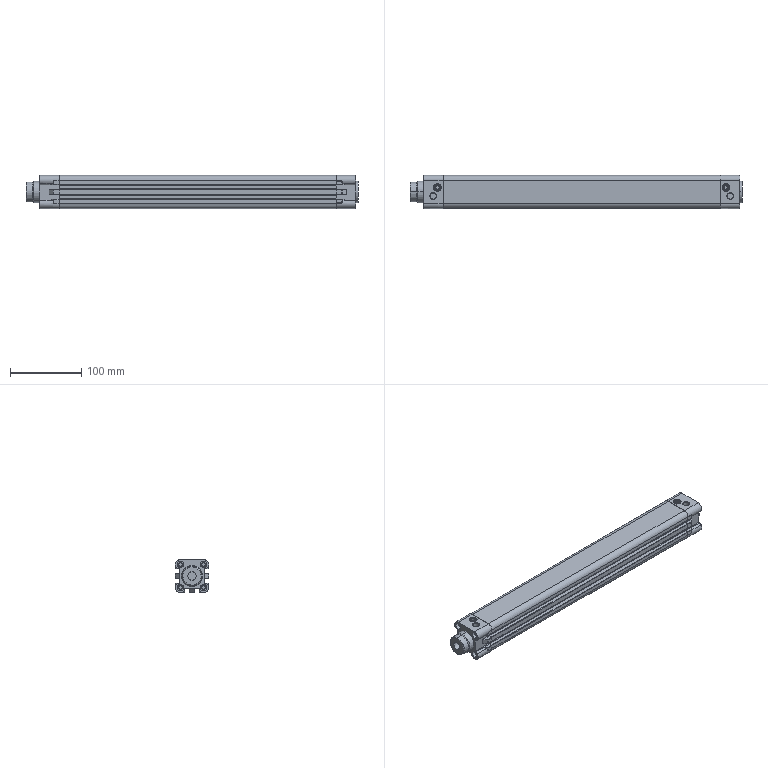Part | SolidWorks | features BaseBody 1 | 1 solid | 398 faces | box 466 x 46.5 x 46.5 mm | volume 520717 mm3 | cylinder 190 | plane 176 | cone 30 | spline 2 | commonest cylinder face diameters 1 x90 4.917 x16 9.4 x16 8 x12 14 x10 15 x10